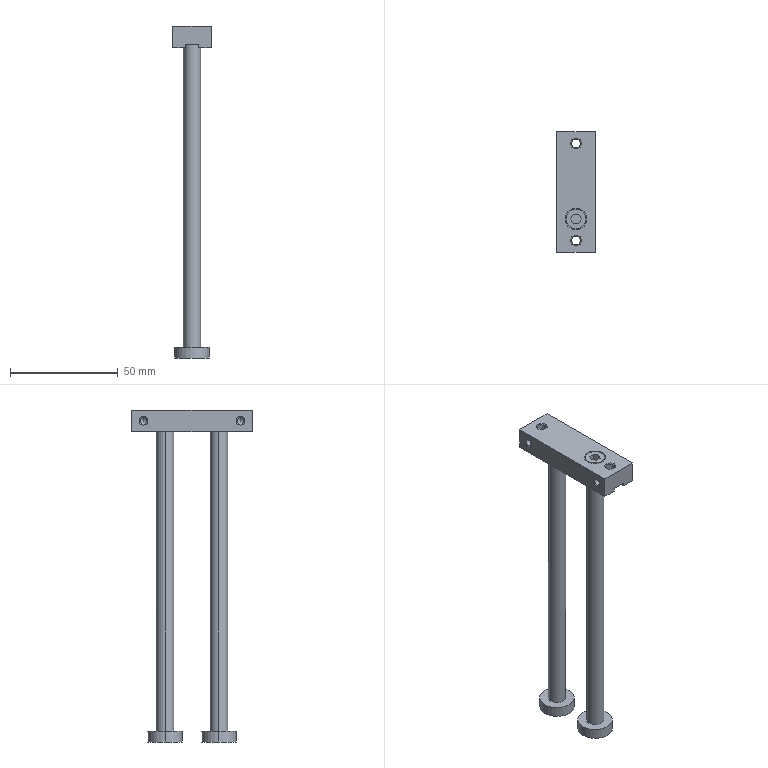Part | SolidWorks | features BaseBody 1 | 1 solid | 90 faces | box 18 x 56 x 154 mm | volume 25127 mm3 | plane 38 | cylinder 28 | cone 24 | commonest cylinder face diameters 3.242 x8 4.134 x4 8 x4 16 x4 5 x2 6 x2